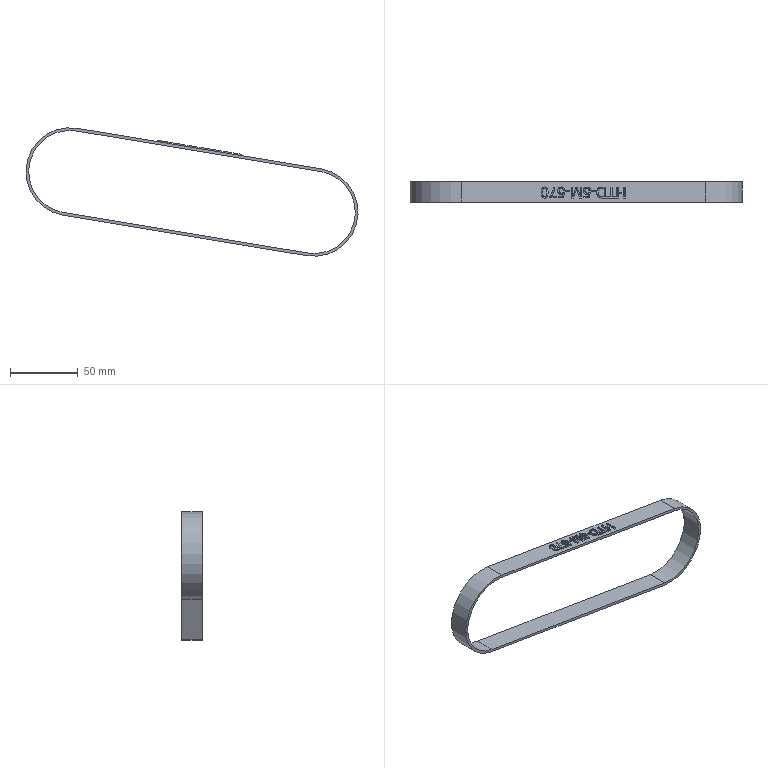Part | STEP file | YBQDJ-PD-5 | 1 solid | 125 faces | box 245.482 x 15 x 95 mm | volume 17074 mm3 | plane 79 | other 42 | cylinder 4 | commonest cylinder face diameters 61 x2 65 x2